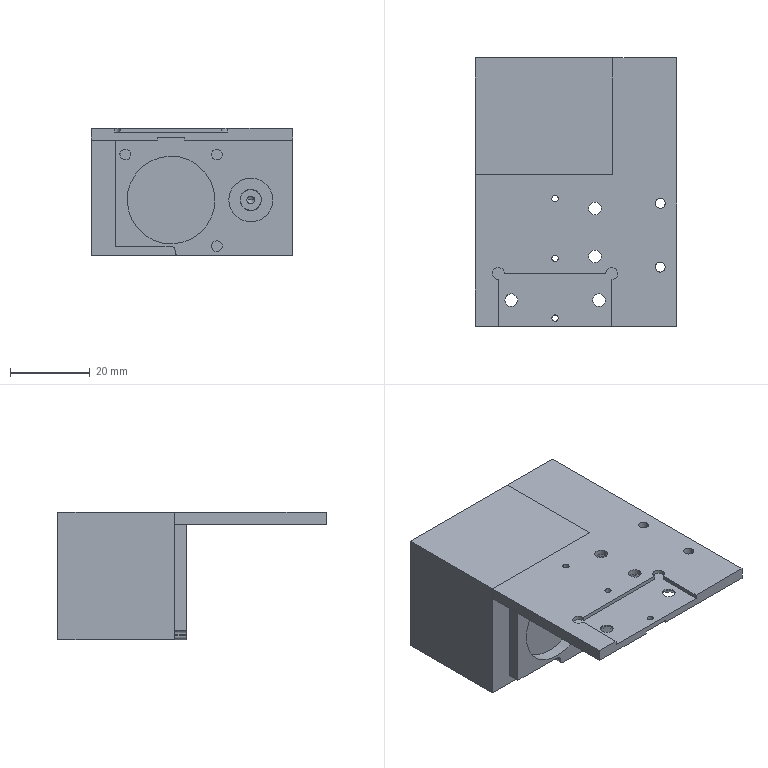Part | 2 solids | 107 faces | box 50.5 x 67.3 x 32 mm | volume 50835 mm3 | spline 73 | plane 34